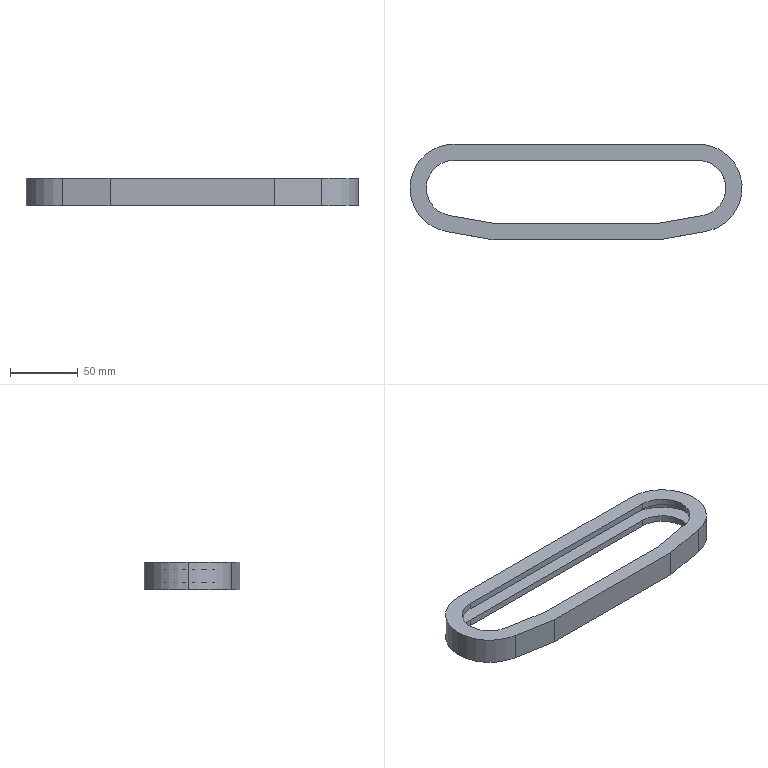Part | SolidWorks | features Extrusion 1, ICE 1 | 1 solid | 32 faces | box 245 x 70.699 x 20 mm | volume 68924 mm3 | plane 20 | cylinder 12 | commonest cylinder face diameters 41 x6 63 x3 65 x3
STEP:
#1=CARTESIAN_POINT('',(121.5,0.,-5.));
#2=VERTEX_POINT('',#1);
#3=CARTESIAN_POINT('',(90.,31.5,-5.));
#4=VERTEX_POINT('',#3);
#5=CARTESIAN_POINT('',(90.,0.,-5.));
#6=DIRECTION('',(0.,0.,1.));
#7=DIRECTION('',(1.,0.,0.));
#8=AXIS2_PLACEMENT_3D('',#5,#6,#7);
#9=CIRCLE('',#8,31.5);
#10=EDGE_CURVE('',#2,#4,#9,.T.);
#11=ORIENTED_EDGE('',*,*,#10,.F.);
#12=CARTESIAN_POINT('',(121.5,0.,5.));
#13=VERTEX_POINT('',#12);
#14=CARTESIAN_POINT('',(121.5,0.,-5.));
#15=DIRECTION('',(0.,0.,1.));
#16=VECTOR('',#15,1000.);
#17=LINE('',#14,#16);
#18=EDGE_CURVE('',#2,#13,#17,.T.);
#19=ORIENTED_EDGE('',*,*,#18,.T.);
#20=CARTESIAN_POINT('',(90.,31.5,5.));
#21=VERTEX_POINT('',#20);
#22=CARTESIAN_POINT('',(90.,0.,5.));
#23=DIRECTION('',(0.,0.,1.));
#24=DIRECTION('',(1.,0.,0.));
#25=AXIS2_PLACEMENT_3D('',#22,#23,#24);
#26=CIRCLE('',#25,31.5);
#27=EDGE_CURVE('',#13,#21,#26,.T.);
#28=ORIENTED_EDGE('',*,*,#27,.T.);
#29=CARTESIAN_POINT('',(90.,31.5,-5.));
#30=DIRECTION('',(0.,0.,1.));
#31=VECTOR('',#30,1000.);
#32=LINE('',#29,#31);
#33=EDGE_CURVE('',#4,#21,#32,.T.);
#34=ORIENTED_EDGE('',*,*,#33,.F.);
#35=EDGE_LOOP('',(#11,#19,#28,#34));
#36=FACE_OUTER_BOUND('',#35,.T.);
#37=CARTESIAN_POINT('',(90.,0.,-5.));
#38=DIRECTION('',(0.,0.,1.));
#39=DIRECTION('',(1.,0.,0.));
#40=AXIS2_PLACEMENT_3D('',#37,#38,#39);
#41=CYLINDRICAL_SURFACE('',#40,31.5);
#42=ADVANCED_FACE('',(#36),#41,.F.);
#43=CARTESIAN_POINT('',(-90.,20.5,10.));
#44=VERTEX_POINT('',#43);
#45=CARTESIAN_POINT('',(-110.5,0.,10.));
#46=VERTEX_POINT('',#45);
#47=CARTESIAN_POINT('',(-90.,0.,10.));
#48=DIRECTION('',(0.,0.,1.));
#49=DIRECTION('',(1.,0.,0.));
#50=AXIS2_PLACEMENT_3D('',#47,#48,#49);
#51=CIRCLE('',#50,20.5);
#52=EDGE_CURVE('',#44,#46,#51,.T.);
#53=ORIENTED_EDGE('',*,*,#52,.T.);
#54=CARTESIAN_POINT('',(-110.5,0.,5.));
#55=VERTEX_POINT('',#54);
#56=CARTESIAN_POINT('',(-110.5,0.,10.));
#57=DIRECTION('',(0.,0.,-1.));
#58=VECTOR('',#57,1000.);
#59=LINE('',#56,#58);
#60=EDGE_CURVE('',#46,#55,#59,.T.);
#61=ORIENTED_EDGE('',*,*,#60,.T.);
#62=CARTESIAN_POINT('',(-90.,20.5,5.));
#63=VERTEX_POINT('',#62);
#64=CARTESIAN_POINT('',(-90.,0.,5.));
#65=DIRECTION('',(0.,0.,1.));
#66=DIRECTION('',(1.,0.,0.));
#67=AXIS2_PLACEMENT_3D('',#64,#65,#66);
#68=CIRCLE('',#67,20.5);
#69=EDGE_CURVE('',#63,#55,#68,.T.);
#70=ORIENTED_EDGE('',*,*,#69,.F.);
#71=CARTESIAN_POINT('',(-90.,20.5,10.));
#72=DIRECTION('',(0.,0.,-1.));
#73=VECTOR('',#72,1000.);
#74=LINE('',#71,#73);
#75=EDGE_CURVE('',#44,#63,#74,.T.);
#76=ORIENTED_EDGE('',*,*,#75,.F.);
#77=EDGE_LOOP('',(#53,#61,#70,#76));
#78=FACE_OUTER_BOUND('',#77,.T.);
#79=CARTESIAN_POINT('',(-90.,0.,10.));
#80=DIRECTION('',(0.,0.,-1.));
#81=DIRECTION('',(-1.,0.,0.));
#82=AXIS2_PLACEMENT_3D('',#79,#80,#81);
#83=CYLINDRICAL_SURFACE('',#82,20.5);
#84=ADVANCED_FACE('',(#78),#83,.F.);
#85=CARTESIAN_POINT('',(-122.5,0.,10.));
#86=VERTEX_POINT('',#85);
#87=CARTESIAN_POINT('',(-95.644,-32.006,10.));
#88=VERTEX_POINT('',#87);
#89=CARTESIAN_POINT('',(-90.,0.,10.));
#90=DIRECTION('',(0.,0.,1.));
#91=DIRECTION('',(1.,0.,0.));
#92=AXIS2_PLACEMENT_3D('',#89,#90,#91);
#93=CIRCLE('',#92,32.5);
#94=EDGE_CURVE('',#86,#88,#93,.T.);
#95=ORIENTED_EDGE('',*,*,#94,.F.);
#96=CARTESIAN_POINT('',(-122.5,0.,-10.));
#97=VERTEX_POINT('',#96);
#98=CARTESIAN_POINT('',(-122.5,0.,10.));
#99=DIRECTION('',(0.,0.,-1.));
#100=VECTOR('',#99,1000.);
#101=LINE('',#98,#100);
#102=EDGE_CURVE('',#86,#97,#101,.T.);
#103=ORIENTED_EDGE('',*,*,#102,.T.);
#104=CARTESIAN_POINT('',(-95.644,-32.006,-10.));
#105=VERTEX_POINT('',#104);
#106=CARTESIAN_POINT('',(-90.,0.,-10.));
#107=DIRECTION('',(0.,0.,1.));
#108=DIRECTION('',(1.,0.,0.));
#109=AXIS2_PLACEMENT_3D('',#106,#107,#108);
#110=CIRCLE('',#109,32.5);
#111=EDGE_CURVE('',#97,#105,#110,.T.);
#112=ORIENTED_EDGE('',*,*,#111,.T.);
#113=CARTESIAN_POINT('',(-95.644,-32.006,10.));
#114=DIRECTION('',(0.,0.,-1.));
#115=VECTOR('',#114,1000.);
#116=LINE('',#113,#115);
#117=EDGE_CURVE('',#88,#105,#116,.T.);
#118=ORIENTED_EDGE('',*,*,#117,.F.);
#119=EDGE_LOOP('',(#95,#103,#112,#118));
#120=FACE_OUTER_BOUND('',#119,.T.);
#121=CARTESIAN_POINT('',(-90.,0.,10.));
#122=DIRECTION('',(0.,0.,-1.));
#123=DIRECTION('',(-1.,0.,0.));
#124=AXIS2_PLACEMENT_3D('',#121,#122,#123);
#125=CYLINDRICAL_SURFACE('',#124,32.5);
#126=ADVANCED_FACE('',(#120),#125,.T.);
#127=CARTESIAN_POINT('',(-90.,20.5,-5.));
#128=VERTEX_POINT('',#127);
#129=CARTESIAN_POINT('',(-110.5,0.,-5.));
#130=VERTEX_POINT('',#129);
#131=CARTESIAN_POINT('',(-90.,0.,-5.));
#132=DIRECTION('',(0.,0.,1.));
#133=DIRECTION('',(1.,0.,0.));
#134=AXIS2_PLACEMENT_3D('',#131,#132,#133);
#135=CIRCLE('',#134,20.5);
#136=EDGE_CURVE('',#128,#130,#135,.T.);
#137=ORIENTED_EDGE('',*,*,#136,.T.);
#138=CARTESIAN_POINT('',(-110.5,0.,-10.));
#139=VERTEX_POINT('',#138);
#140=CARTESIAN_POINT('',(-110.5,0.,10.));
#141=DIRECTION('',(0.,0.,-1.));
#142=VECTOR('',#141,1000.);
#143=LINE('',#140,#142);
#144=EDGE_CURVE('',#130,#139,#143,.T.);
#145=ORIENTED_EDGE('',*,*,#144,.T.);
#146=CARTESIAN_POINT('',(-90.,20.5,-10.));
#147=VERTEX_POINT('',#146);
#148=CARTESIAN_POINT('',(-90.,0.,-10.));
#149=DIRECTION('',(0.,0.,1.));
#150=DIRECTION('',(1.,0.,0.));
#151=AXIS2_PLACEMENT_3D('',#148,#149,#150);
#152=CIRCLE('',#151,20.5);
#153=EDGE_CURVE('',#147,#139,#152,.T.);
#154=ORIENTED_EDGE('',*,*,#153,.F.);
#155=CARTESIAN_POINT('',(-90.,20.5,10.));
#156=DIRECTION('',(0.,0.,-1.));
#157=VECTOR('',#156,1000.);
#158=LINE('',#155,#157);
#159=EDGE_CURVE('',#128,#147,#158,.T.);
#160=ORIENTED_EDGE('',*,*,#159,.F.);
#161=EDGE_LOOP('',(#137,#145,#154,#160));
#162=FACE_OUTER_BOUND('',#161,.T.);
#163=CARTESIAN_POINT('',(-90.,0.,10.));
#164=DIRECTION('',(0.,0.,-1.));
#165=DIRECTION('',(-1.,0.,0.));
#166=AXIS2_PLACEMENT_3D('',#163,#164,#165);
#167=CYLINDRICAL_SURFACE('',#166,20.5);
#168=ADVANCED_FACE('',(#162),#167,.F.);
#169=ORIENTED_EDGE('',*,*,#144,.F.);
#170=CARTESIAN_POINT('',(-93.56,-20.189,-5.));
#171=VERTEX_POINT('',#170);
#172=CARTESIAN_POINT('',(-90.,0.,-5.));
#173=DIRECTION('',(0.,0.,1.));
#174=DIRECTION('',(1.,0.,0.));
#175=AXIS2_PLACEMENT_3D('',#172,#173,#174);
#176=CIRCLE('',#175,20.5);
#177=EDGE_CURVE('',#130,#171,#176,.T.);
#178=ORIENTED_EDGE('',*,*,#177,.T.);
#179=CARTESIAN_POINT('',(-93.56,-20.189,-10.));
#180=VERTEX_POINT('',#179);
#181=CARTESIAN_POINT('',(-93.56,-20.189,10.));
#182=DIRECTION('',(0.,0.,-1.));
#183=VECTOR('',#182,1000.);
#184=LINE('',#181,#183);
#185=EDGE_CURVE('',#171,#180,#184,.T.);
#186=ORIENTED_EDGE('',*,*,#185,.T.);
#187=CARTESIAN_POINT('',(-90.,0.,-10.));
#188=DIRECTION('',(0.,0.,1.));
#189=DIRECTION('',(1.,0.,0.));
#190=AXIS2_PLACEMENT_3D('',#187,#188,#189);
#191=CIRCLE('',#190,20.5);
#192=EDGE_CURVE('',#139,#180,#191,.T.);
#193=ORIENTED_EDGE('',*,*,#192,.F.);
#194=EDGE_LOOP('',(#169,#178,#186,#193));
#195=FACE_OUTER_BOUND('',#194,.T.);
#196=CARTESIAN_POINT('',(-90.,0.,10.));
#197=DIRECTION('',(0.,0.,-1.));
#198=DIRECTION('',(-1.,0.,0.));
#199=AXIS2_PLACEMENT_3D('',#196,#197,#198);
#200=CYLINDRICAL_SURFACE('',#199,20.5);
#201=ADVANCED_FACE('',(#195),#200,.F.);
#202=ORIENTED_EDGE('',*,*,#185,.F.);
#203=CARTESIAN_POINT('',(-59.475,-26.199,-5.));
#204=VERTEX_POINT('',#203);
#205=CARTESIAN_POINT('',(-59.475,-26.199,-5.));
#206=DIRECTION('',(0.9848,-0.1736,0.));
#207=VECTOR('',#206,1000.);
#208=LINE('',#205,#207);
#209=EDGE_CURVE('',#171,#204,#208,.T.);
#210=ORIENTED_EDGE('',*,*,#209,.T.);
#211=CARTESIAN_POINT('',(-59.475,-26.199,-10.));
#212=VERTEX_POINT('',#211);
#213=CARTESIAN_POINT('',(-59.475,-26.199,10.));
#214=DIRECTION('',(0.,0.,-1.));
#215=VECTOR('',#214,1000.);
#216=LINE('',#213,#215);
#217=EDGE_CURVE('',#204,#212,#216,.T.);
#218=ORIENTED_EDGE('',*,*,#217,.T.);
#219=CARTESIAN_POINT('',(-59.475,-26.199,-10.));
#220=DIRECTION('',(0.9848,-0.1736,0.));
#221=VECTOR('',#220,1000.);
#222=LINE('',#219,#221);
#223=EDGE_CURVE('',#180,#212,#222,.T.);
#224=ORIENTED_EDGE('',*,*,#223,.F.);
#225=EDGE_LOOP('',(#202,#210,#218,#224));
#226=FACE_OUTER_BOUND('',#225,.T.);
#227=CARTESIAN_POINT('',(-59.475,-26.199,10.));
#228=DIRECTION('',(0.1736,0.9848,0.));
#229=DIRECTION('',(-0.9848,0.1736,0.));
#230=AXIS2_PLACEMENT_3D('',#227,#228,#229);
#231=PLANE('',#230);
#232=ADVANCED_FACE('',(#226),#231,.T.);
#233=ORIENTED_EDGE('',*,*,#217,.F.);
#234=CARTESIAN_POINT('',(59.475,-26.199,-5.));
#235=VERTEX_POINT('',#234);
#236=CARTESIAN_POINT('',(-59.475,-26.199,-5.));
#237=DIRECTION('',(1.,0.,0.));
#238=VECTOR('',#237,1000.);
#239=LINE('',#236,#238);
#240=EDGE_CURVE('',#204,#235,#239,.T.);
#241=ORIENTED_EDGE('',*,*,#240,.T.);
#242=CARTESIAN_POINT('',(59.475,-26.199,-10.));
#243=VERTEX_POINT('',#242);
#244=CARTESIAN_POINT('',(59.475,-26.199,10.));
#245=DIRECTION('',(0.,0.,-1.));
#246=VECTOR('',#245,1000.);
#247=LINE('',#244,#246);
#248=EDGE_CURVE('',#235,#243,#247,.T.);
#249=ORIENTED_EDGE('',*,*,#248,.T.);
#250=CARTESIAN_POINT('',(-59.475,-26.199,-10.));
#251=DIRECTION('',(1.,0.,0.));
#252=VECTOR('',#251,1000.);
#253=LINE('',#250,#252);
#254=EDGE_CURVE('',#212,#243,#253,.T.);
#255=ORIENTED_EDGE('',*,*,#254,.F.);
#256=EDGE_LOOP('',(#233,#241,#249,#255));
#257=FACE_OUTER_BOUND('',#256,.T.);
#258=CARTESIAN_POINT('',(-59.475,-26.199,10.));
#259=DIRECTION('',(0.,1.,0.));
#260=DIRECTION('',(0.,0.,1.));
#261=AXIS2_PLACEMENT_3D('',#258,#259,#260);
#262=PLANE('',#261);
#263=ADVANCED_FACE('',(#257),#262,.T.);
#264=ORIENTED_EDGE('',*,*,#248,.F.);
#265=CARTESIAN_POINT('',(93.56,-20.189,-5.));
#266=VERTEX_POINT('',#265);
#267=CARTESIAN_POINT('',(59.475,-26.199,-5.));
#268=DIRECTION('',(0.9848,0.1736,0.));
#269=VECTOR('',#268,1000.);
#270=LINE('',#267,#269);
#271=EDGE_CURVE('',#235,#266,#270,.T.);
#272=ORIENTED_EDGE('',*,*,#271,.T.);
#273=CARTESIAN_POINT('',(93.56,-20.189,-10.));
#274=VERTEX_POINT('',#273);
#275=CARTESIAN_POINT('',(93.56,-20.189,10.));
#276=DIRECTION('',(0.,0.,-1.));
#277=VECTOR('',#276,1000.);
#278=LINE('',#275,#277);
#279=EDGE_CURVE('',#266,#274,#278,.T.);
#280=ORIENTED_EDGE('',*,*,#279,.T.);
#281=CARTESIAN_POINT('',(59.475,-26.199,-10.));
#282=DIRECTION('',(0.9848,0.1736,0.));
#283=VECTOR('',#282,1000.);
#284=LINE('',#281,#283);
#285=EDGE_CURVE('',#243,#274,#284,.T.);
#286=ORIENTED_EDGE('',*,*,#285,.F.);
#287=EDGE_LOOP('',(#264,#272,#280,#286));
#288=FACE_OUTER_BOUND('',#287,.T.);
#289=CARTESIAN_POINT('',(59.475,-26.199,10.));
#290=DIRECTION('',(-0.1736,0.9848,0.));
#291=DIRECTION('',(-0.9848,-0.1736,0.));
#292=AXIS2_PLACEMENT_3D('',#289,#290,#291);
#293=PLANE('',#292);
#294=ADVANCED_FACE('',(#288),#293,.T.);
#295=ORIENTED_EDGE('',*,*,#279,.F.);
#296=CARTESIAN_POINT('',(90.,20.5,-5.));
#297=VERTEX_POINT('',#296);
#298=CARTESIAN_POINT('',(90.,0.,-5.));
#299=DIRECTION('',(0.,0.,1.));
#300=DIRECTION('',(1.,0.,0.));
#301=AXIS2_PLACEMENT_3D('',#298,#299,#300);
#302=CIRCLE('',#301,20.5);
#303=EDGE_CURVE('',#266,#297,#302,.T.);
#304=ORIENTED_EDGE('',*,*,#303,.T.);
#305=CARTESIAN_POINT('',(90.,20.5,-10.));
#306=VERTEX_POINT('',#305);
#307=CARTESIAN_POINT('',(90.,20.5,10.));
#308=DIRECTION('',(0.,0.,-1.));
#309=VECTOR('',#308,1000.);
#310=LINE('',#307,#309);
#311=EDGE_CURVE('',#297,#306,#310,.T.);
#312=ORIENTED_EDGE('',*,*,#311,.T.);
#313=CARTESIAN_POINT('',(90.,0.,-10.));
#314=DIRECTION('',(0.,0.,1.));
#315=DIRECTION('',(-1.,0.,0.));
#316=AXIS2_PLACEMENT_3D('',#313,#314,#315);
#317=CIRCLE('',#316,20.5);
#318=EDGE_CURVE('',#274,#306,#317,.T.);
#319=ORIENTED_EDGE('',*,*,#318,.F.);
#320=EDGE_LOOP('',(#295,#304,#312,#319));
#321=FACE_OUTER_BOUND('',#320,.T.);
#322=CARTESIAN_POINT('',(90.,0.,10.));
#323=DIRECTION('',(0.,0.,-1.));
#324=DIRECTION('',(-1.,0.,0.));
#325=AXIS2_PLACEMENT_3D('',#322,#323,#324);
#326=CYLINDRICAL_SURFACE('',#325,20.5);
#327=ADVANCED_FACE('',(#321),#326,.F.);
#328=ORIENTED_EDGE('',*,*,#311,.F.);
#329=CARTESIAN_POINT('',(-90.,20.5,-5.));
#330=DIRECTION('',(-1.,0.,0.));
#331=VECTOR('',#330,1000.);
#332=LINE('',#329,#331);
#333=EDGE_CURVE('',#297,#128,#332,.T.);
#334=ORIENTED_EDGE('',*,*,#333,.T.);
#335=ORIENTED_EDGE('',*,*,#159,.T.);
#336=CARTESIAN_POINT('',(-90.,20.5,-10.));
#337=DIRECTION('',(-1.,0.,0.));
#338=VECTOR('',#337,1000.);
#339=LINE('',#336,#338);
#340=EDGE_CURVE('',#306,#147,#339,.T.);
#341=ORIENTED_EDGE('',*,*,#340,.F.);
#342=EDGE_LOOP('',(#328,#334,#335,#341));
#343=FACE_OUTER_BOUND('',#342,.T.);
#344=CARTESIAN_POINT('',(-90.,20.5,10.));
#345=DIRECTION('',(0.,-1.,0.));
#346=DIRECTION('',(0.,0.,-1.));
#347=AXIS2_PLACEMENT_3D('',#344,#345,#346);
#348=PLANE('',#347);
#349=ADVANCED_FACE('',(#343),#348,.T.);
#350=CARTESIAN_POINT('',(-90.,32.5,10.));
#351=VERTEX_POINT('',#350);
#352=CARTESIAN_POINT('',(-90.,0.,10.));
#353=DIRECTION('',(0.,0.,1.));
#354=DIRECTION('',(1.,0.,0.));
#355=AXIS2_PLACEMENT_3D('',#352,#353,#354);
#356=CIRCLE('',#355,32.5);
#357=EDGE_CURVE('',#351,#86,#356,.T.);
#358=ORIENTED_EDGE('',*,*,#357,.T.);
#359=ORIENTED_EDGE('',*,*,#94,.T.);
#360=CARTESIAN_POINT('',(-60.525,-38.199,10.));
#361=VERTEX_POINT('',#360);
#362=CARTESIAN_POINT('',(-60.525,-38.199,10.));
#363=DIRECTION('',(0.9848,-0.1736,0.));
#364=VECTOR('',#363,1000.);
#365=LINE('',#362,#364);
#366=EDGE_CURVE('',#88,#361,#365,.T.);
#367=ORIENTED_EDGE('',*,*,#366,.T.);
#368=CARTESIAN_POINT('',(60.525,-38.199,10.));
#369=VERTEX_POINT('',#368);
#370=CARTESIAN_POINT('',(-60.525,-38.199,10.));
#371=DIRECTION('',(1.,0.,0.));
#372=VECTOR('',#371,1000.);
#373=LINE('',#370,#372);
#374=EDGE_CURVE('',#361,#369,#373,.T.);
#375=ORIENTED_EDGE('',*,*,#374,.T.);
#376=CARTESIAN_POINT('',(95.644,-32.006,10.));
#377=VERTEX_POINT('',#376);
#378=CARTESIAN_POINT('',(60.525,-38.199,10.));
#379=DIRECTION('',(0.9848,0.1736,0.));
#380=VECTOR('',#379,1000.);
#381=LINE('',#378,#380);
#382=EDGE_CURVE('',#369,#377,#381,.T.);
#383=ORIENTED_EDGE('',*,*,#382,.T.);
#384=CARTESIAN_POINT('',(90.,32.5,10.));
#385=VERTEX_POINT('',#384);
#386=CARTESIAN_POINT('',(90.,0.,10.));
#387=DIRECTION('',(0.,0.,1.));
#388=DIRECTION('',(-1.,0.,0.));
#389=AXIS2_PLACEMENT_3D('',#386,#387,#388);
#390=CIRCLE('',#389,32.5);
#391=EDGE_CURVE('',#377,#385,#390,.T.);
#392=ORIENTED_EDGE('',*,*,#391,.T.);
#393=CARTESIAN_POINT('',(-90.,32.5,10.));
#394=DIRECTION('',(-1.,0.,0.));
#395=VECTOR('',#394,1000.);
#396=LINE('',#393,#395);
#397=EDGE_CURVE('',#385,#351,#396,.T.);
#398=ORIENTED_EDGE('',*,*,#397,.T.);
#399=EDGE_LOOP('',(#358,#359,#367,#375,#383,#392,#398));
#400=FACE_OUTER_BOUND('',#399,.T.);
#401=CARTESIAN_POINT('',(-93.56,-20.189,10.));
#402=VERTEX_POINT('',#401);
#403=CARTESIAN_POINT('',(-59.475,-26.199,10.));
#404=VERTEX_POINT('',#403);
#405=CARTESIAN_POINT('',(-59.475,-26.199,10.));
#406=DIRECTION('',(0.9848,-0.1736,0.));
#407=VECTOR('',#406,1000.);
#408=LINE('',#405,#407);
#409=EDGE_CURVE('',#402,#404,#408,.T.);
#410=ORIENTED_EDGE('',*,*,#409,.F.);
#411=CARTESIAN_POINT('',(-90.,0.,10.));
#412=DIRECTION('',(0.,0.,1.));
#413=DIRECTION('',(1.,0.,0.));
#414=AXIS2_PLACEMENT_3D('',#411,#412,#413);
#415=CIRCLE('',#414,20.5);
#416=EDGE_CURVE('',#46,#402,#415,.T.);
#417=ORIENTED_EDGE('',*,*,#416,.F.);
#418=ORIENTED_EDGE('',*,*,#52,.F.);
#419=CARTESIAN_POINT('',(90.,20.5,10.));
#420=VERTEX_POINT('',#419);
#421=CARTESIAN_POINT('',(-90.,20.5,10.));
#422=DIRECTION('',(-1.,0.,0.));
#423=VECTOR('',#422,1000.);
#424=LINE('',#421,#423);
#425=EDGE_CURVE('',#420,#44,#424,.T.);
#426=ORIENTED_EDGE('',*,*,#425,.F.);
#427=CARTESIAN_POINT('',(93.56,-20.189,10.));
#428=VERTEX_POINT('',#427);
#429=CARTESIAN_POINT('',(90.,0.,10.));
#430=DIRECTION('',(0.,0.,1.));
#431=DIRECTION('',(-1.,0.,0.));
#432=AXIS2_PLACEMENT_3D('',#429,#430,#431);
#433=CIRCLE('',#432,20.5);
#434=EDGE_CURVE('',#428,#420,#433,.T.);
#435=ORIENTED_EDGE('',*,*,#434,.F.);
#436=CARTESIAN_POINT('',(59.475,-26.199,10.));
#437=VERTEX_POINT('',#436);
#438=CARTESIAN_POINT('',(59.475,-26.199,10.));
#439=DIRECTION('',(0.9848,0.1736,0.));
#440=VECTOR('',#439,1000.);
#441=LINE('',#438,#440);
#442=EDGE_CURVE('',#437,#428,#441,.T.);
#443=ORIENTED_EDGE('',*,*,#442,.F.);
#444=CARTESIAN_POINT('',(-59.475,-26.199,10.));
#445=DIRECTION('',(1.,0.,0.));
#446=VECTOR('',#445,1000.);
#447=LINE('',#444,#446);
#448=EDGE_CURVE('',#404,#437,#447,.T.);
#449=ORIENTED_EDGE('',*,*,#448,.F.);
#450=EDGE_LOOP('',(#410,#417,#418,#426,#435,#443,#449));
#451=FACE_BOUND('',#450,.T.);
#452=CARTESIAN_POINT('',(-90.,0.,10.));
#453=DIRECTION('',(0.,0.,1.));
#454=DIRECTION('',(1.,0.,0.));
#455=AXIS2_PLACEMENT_3D('',#452,#453,#454);
#456=PLANE('',#455);
#457=ADVANCED_FACE('',(#400,#451),#456,.T.);
#458=CARTESIAN_POINT('',(-90.,32.5,-10.));
#459=VERTEX_POINT('',#458);
#460=CARTESIAN_POINT('',(-90.,0.,-10.));
#461=DIRECTION('',(0.,0.,1.));
#462=DIRECTION('',(1.,0.,0.));
#463=AXIS2_PLACEMENT_3D('',#460,#461,#462);
#464=CIRCLE('',#463,32.5);
#465=EDGE_CURVE('',#459,#97,#464,.T.);
#466=ORIENTED_EDGE('',*,*,#465,.F.);
#467=CARTESIAN_POINT('',(90.,32.5,-10.));
#468=VERTEX_POINT('',#467);
#469=CARTESIAN_POINT('',(-90.,32.5,-10.));
#470=DIRECTION('',(-1.,0.,0.));
#471=VECTOR('',#470,1000.);
#472=LINE('',#469,#471);
#473=EDGE_CURVE('',#468,#459,#472,.T.);
#474=ORIENTED_EDGE('',*,*,#473,.F.);
#475=CARTESIAN_POINT('',(95.644,-32.006,-10.));
#476=VERTEX_POINT('',#475);
#477=CARTESIAN_POINT('',(90.,0.,-10.));
#478=DIRECTION('',(0.,0.,1.));
#479=DIRECTION('',(-1.,0.,0.));
#480=AXIS2_PLACEMENT_3D('',#477,#478,#479);
#481=CIRCLE('',#480,32.5);
#482=EDGE_CURVE('',#476,#468,#481,.T.);
#483=ORIENTED_EDGE('',*,*,#482,.F.);
#484=CARTESIAN_POINT('',(60.525,-38.199,-10.));
#485=VERTEX_POINT('',#484);
#486=CARTESIAN_POINT('',(60.525,-38.199,-10.));
#487=DIRECTION('',(0.9848,0.1736,0.));
#488=VECTOR('',#487,1000.);
#489=LINE('',#486,#488);
#490=EDGE_CURVE('',#485,#476,#489,.T.);
#491=ORIENTED_EDGE('',*,*,#490,.F.);
#492=CARTESIAN_POINT('',(-60.525,-38.199,-10.));
#493=VERTEX_POINT('',#492);
#494=CARTESIAN_POINT('',(-60.525,-38.199,-10.));
#495=DIRECTION('',(1.,0.,0.));
#496=VECTOR('',#495,1000.);
#497=LINE('',#494,#496);
#498=EDGE_CURVE('',#493,#485,#497,.T.);
#499=ORIENTED_EDGE('',*,*,#498,.F.);
#500=CARTESIAN_POINT('',(-60.525,-38.199,-10.));
#501=DIRECTION('',(0.9848,-0.1736,0.));
#502=VECTOR('',#501,1000.);
#503=LINE('',#500,#502);
#504=EDGE_CURVE('',#105,#493,#503,.T.);
#505=ORIENTED_EDGE('',*,*,#504,.F.);
#506=ORIENTED_EDGE('',*,*,#111,.F.);
#507=EDGE_LOOP('',(#466,#474,#483,#491,#499,#505,#506));
#508=FACE_OUTER_BOUND('',#507,.T.);
#509=ORIENTED_EDGE('',*,*,#153,.T.);
#510=ORIENTED_EDGE('',*,*,#192,.T.);
#511=ORIENTED_EDGE('',*,*,#223,.T.);
#512=ORIENTED_EDGE('',*,*,#254,.T.);
#513=ORIENTED_EDGE('',*,*,#285,.T.);
#514=ORIENTED_EDGE('',*,*,#318,.T.);
#515=ORIENTED_EDGE('',*,*,#340,.T.);
#516=EDGE_LOOP('',(#509,#510,#511,#512,#513,#514,#515));
#517=FACE_BOUND('',#516,.T.);
#518=CARTESIAN_POINT('',(-90.,0.,-10.));
#519=DIRECTION('',(0.,0.,1.));
#520=DIRECTION('',(1.,0.,0.));
#521=AXIS2_PLACEMENT_3D('',#518,#519,#520);
#522=PLANE('',#521);
#523=ADVANCED_FACE('',(#508,#517),#522,.F.);
#524=ORIENTED_EDGE('',*,*,#102,.F.);
#525=ORIENTED_EDGE('',*,*,#357,.F.);
#526=CARTESIAN_POINT('',(-90.,32.5,10.));
#527=DIRECTION('',(0.,0.,-1.));
#528=VECTOR('',#527,1000.);
#529=LINE('',#526,#528);
#530=EDGE_CURVE('',#351,#459,#529,.T.);
#531=ORIENTED_EDGE('',*,*,#530,.T.);
#532=ORIENTED_EDGE('',*,*,#465,.T.);
#533=EDGE_LOOP('',(#524,#525,#531,#532));
#534=FACE_OUTER_BOUND('',#533,.T.);
#535=CARTESIAN_POINT('',(-90.,0.,10.));
#536=DIRECTION('',(0.,0.,-1.));
#537=DIRECTION('',(-1.,0.,0.));
#538=AXIS2_PLACEMENT_3D('',#535,#536,#537);
#539=CYLINDRICAL_SURFACE('',#538,32.5);
#540=ADVANCED_FACE('',(#534),#539,.T.);
#541=ORIENTED_EDGE('',*,*,#504,.T.);
#542=CARTESIAN_POINT('',(-60.525,-38.199,10.));
#543=DIRECTION('',(0.,0.,-1.));
#544=VECTOR('',#543,1000.);
#545=LINE('',#542,#544);
#546=EDGE_CURVE('',#361,#493,#545,.T.);
#547=ORIENTED_EDGE('',*,*,#546,.F.);
#548=ORIENTED_EDGE('',*,*,#366,.F.);
#549=ORIENTED_EDGE('',*,*,#117,.T.);
#550=EDGE_LOOP('',(#541,#547,#548,#549));
#551=FACE_OUTER_BOUND('',#550,.T.);
#552=CARTESIAN_POINT('',(-60.525,-38.199,10.));
#553=DIRECTION('',(0.1736,0.9848,0.));
#554=DIRECTION('',(-0.9848,0.1736,0.));
#555=AXIS2_PLACEMENT_3D('',#552,#553,#554);
#556=PLANE('',#555);
#557=ADVANCED_FACE('',(#551),#556,.F.);
#558=ORIENTED_EDGE('',*,*,#498,.T.);
#559=CARTESIAN_POINT('',(60.525,-38.199,10.));
#560=DIRECTION('',(0.,0.,-1.));
#561=VECTOR('',#560,1000.);
#562=LINE('',#559,#561);
#563=EDGE_CURVE('',#369,#485,#562,.T.);
#564=ORIENTED_EDGE('',*,*,#563,.F.);
#565=ORIENTED_EDGE('',*,*,#374,.F.);
#566=ORIENTED_EDGE('',*,*,#546,.T.);
#567=EDGE_LOOP('',(#558,#564,#565,#566));
#568=FACE_OUTER_BOUND('',#567,.T.);
#569=CARTESIAN_POINT('',(-60.525,-38.199,10.));
#570=DIRECTION('',(0.,1.,0.));
#571=DIRECTION('',(0.,0.,1.));
#572=AXIS2_PLACEMENT_3D('',#569,#570,#571);
#573=PLANE('',#572);
#574=ADVANCED_FACE('',(#568),#573,.F.);
#575=ORIENTED_EDGE('',*,*,#490,.T.);
#576=CARTESIAN_POINT('',(95.644,-32.006,10.));
#577=DIRECTION('',(0.,0.,-1.));
#578=VECTOR('',#577,1000.);
#579=LINE('',#576,#578);
#580=EDGE_CURVE('',#377,#476,#579,.T.);
#581=ORIENTED_EDGE('',*,*,#580,.F.);
#582=ORIENTED_EDGE('',*,*,#382,.F.);
#583=ORIENTED_EDGE('',*,*,#563,.T.);
#584=EDGE_LOOP('',(#575,#581,#582,#583));
#585=FACE_OUTER_BOUND('',#584,.T.);
#586=CARTESIAN_POINT('',(60.525,-38.199,10.));
#587=DIRECTION('',(-0.1736,0.9848,0.));
#588=DIRECTION('',(-0.9848,-0.1736,0.));
#589=AXIS2_PLACEMENT_3D('',#586,#587,#588);
#590=PLANE('',#589);
#591=ADVANCED_FACE('',(#585),#590,.F.);
#592=ORIENTED_EDGE('',*,*,#482,.T.);
#593=CARTESIAN_POINT('',(90.,32.5,10.));
#594=DIRECTION('',(0.,0.,-1.));
#595=VECTOR('',#594,1000.);
#596=LINE('',#593,#595);
#597=EDGE_CURVE('',#385,#468,#596,.T.);
#598=ORIENTED_EDGE('',*,*,#597,.F.);
#599=ORIENTED_EDGE('',*,*,#391,.F.);
#600=ORIENTED_EDGE('',*,*,#580,.T.);
#601=EDGE_LOOP('',(#592,#598,#599,#600));
#602=FACE_OUTER_BOUND('',#601,.T.);
#603=CARTESIAN_POINT('',(90.,0.,10.));
#604=DIRECTION('',(0.,0.,-1.));
#605=DIRECTION('',(-1.,0.,0.));
#606=AXIS2_PLACEMENT_3D('',#603,#604,#605);
#607=CYLINDRICAL_SURFACE('',#606,32.5);
#608=ADVANCED_FACE('',(#602),#607,.T.);
#609=ORIENTED_EDGE('',*,*,#473,.T.);
#610=ORIENTED_EDGE('',*,*,#530,.F.);
#611=ORIENTED_EDGE('',*,*,#397,.F.);
#612=ORIENTED_EDGE('',*,*,#597,.T.);
#613=EDGE_LOOP('',(#609,#610,#611,#612));
#614=FACE_OUTER_BOUND('',#613,.T.);
#615=CARTESIAN_POINT('',(-90.,32.5,10.));
#616=DIRECTION('',(0.,-1.,0.));
#617=DIRECTION('',(0.,0.,-1.));
#618=AXIS2_PLACEMENT_3D('',#615,#616,#617);
#619=PLANE('',#618);
#620=ADVANCED_FACE('',(#614),#619,.F.);
#621=ORIENTED_EDGE('',*,*,#60,.F.);
#622=ORIENTED_EDGE('',*,*,#416,.T.);
#623=CARTESIAN_POINT('',(-93.56,-20.189,5.));
#624=VERTEX_POINT('',#623);
#625=CARTESIAN_POINT('',(-93.56,-20.189,10.));
#626=DIRECTION('',(0.,0.,-1.));
#627=VECTOR('',#626,1000.);
#628=LINE('',#625,#627);
#629=EDGE_CURVE('',#402,#624,#628,.T.);
#630=ORIENTED_EDGE('',*,*,#629,.T.);
#631=CARTESIAN_POINT('',(-90.,0.,5.));
#632=DIRECTION('',(0.,0.,1.));
#633=DIRECTION('',(1.,0.,0.));
#634=AXIS2_PLACEMENT_3D('',#631,#632,#633);
#635=CIRCLE('',#634,20.5);
#636=EDGE_CURVE('',#55,#624,#635,.T.);
#637=ORIENTED_EDGE('',*,*,#636,.F.);
#638=EDGE_LOOP('',(#621,#622,#630,#637));
#639=FACE_OUTER_BOUND('',#638,.T.);
#640=CARTESIAN_POINT('',(-90.,0.,10.));
#641=DIRECTION('',(0.,0.,-1.));
#642=DIRECTION('',(-1.,0.,0.));
#643=AXIS2_PLACEMENT_3D('',#640,#641,#642);
#644=CYLINDRICAL_SURFACE('',#643,20.5);
#645=ADVANCED_FACE('',(#639),#644,.F.);
#646=CARTESIAN_POINT('',(-59.475,-26.199,5.));
#647=VERTEX_POINT('',#646);
#648=CARTESIAN_POINT('',(-59.475,-26.199,5.));
#649=DIRECTION('',(0.9848,-0.1736,0.));
#650=VECTOR('',#649,1000.);
#651=LINE('',#648,#650);
#652=EDGE_CURVE('',#624,#647,#651,.T.);
#653=ORIENTED_EDGE('',*,*,#652,.F.);
#654=ORIENTED_EDGE('',*,*,#629,.F.);
#655=ORIENTED_EDGE('',*,*,#409,.T.);
#656=CARTESIAN_POINT('',(-59.475,-26.199,10.));
#657=DIRECTION('',(0.,0.,-1.));
#658=VECTOR('',#657,1000.);
#659=LINE('',#656,#658);
#660=EDGE_CURVE('',#404,#647,#659,.T.);
#661=ORIENTED_EDGE('',*,*,#660,.T.);
#662=EDGE_LOOP('',(#653,#654,#655,#661));
#663=FACE_OUTER_BOUND('',#662,.T.);
#664=CARTESIAN_POINT('',(-59.475,-26.199,10.));
#665=DIRECTION('',(0.1736,0.9848,0.));
#666=DIRECTION('',(-0.9848,0.1736,0.));
#667=AXIS2_PLACEMENT_3D('',#664,#665,#666);
#668=PLANE('',#667);
#669=ADVANCED_FACE('',(#663),#668,.T.);
#670=CARTESIAN_POINT('',(59.475,-26.199,5.));
#671=VERTEX_POINT('',#670);
#672=CARTESIAN_POINT('',(-59.475,-26.199,5.));
#673=DIRECTION('',(1.,0.,0.));
#674=VECTOR('',#673,1000.);
#675=LINE('',#672,#674);
#676=EDGE_CURVE('',#647,#671,#675,.T.);
#677=ORIENTED_EDGE('',*,*,#676,.F.);
#678=ORIENTED_EDGE('',*,*,#660,.F.);
#679=ORIENTED_EDGE('',*,*,#448,.T.);
#680=CARTESIAN_POINT('',(59.475,-26.199,10.));
#681=DIRECTION('',(0.,0.,-1.));
#682=VECTOR('',#681,1000.);
#683=LINE('',#680,#682);
#684=EDGE_CURVE('',#437,#671,#683,.T.);
#685=ORIENTED_EDGE('',*,*,#684,.T.);
#686=EDGE_LOOP('',(#677,#678,#679,#685));
#687=FACE_OUTER_BOUND('',#686,.T.);
#688=CARTESIAN_POINT('',(-59.475,-26.199,10.));
#689=DIRECTION('',(0.,1.,0.));
#690=DIRECTION('',(0.,0.,1.));
#691=AXIS2_PLACEMENT_3D('',#688,#689,#690);
#692=PLANE('',#691);
#693=ADVANCED_FACE('',(#687),#692,.T.);
#694=CARTESIAN_POINT('',(93.56,-20.189,5.));
#695=VERTEX_POINT('',#694);
#696=CARTESIAN_POINT('',(59.475,-26.199,5.));
#697=DIRECTION('',(0.9848,0.1736,0.));
#698=VECTOR('',#697,1000.);
#699=LINE('',#696,#698);
#700=EDGE_CURVE('',#671,#695,#699,.T.);
#701=ORIENTED_EDGE('',*,*,#700,.F.);
#702=ORIENTED_EDGE('',*,*,#684,.F.);
#703=ORIENTED_EDGE('',*,*,#442,.T.);
#704=CARTESIAN_POINT('',(93.56,-20.189,10.));
#705=DIRECTION('',(0.,0.,-1.));
#706=VECTOR('',#705,1000.);
#707=LINE('',#704,#706);
#708=EDGE_CURVE('',#428,#695,#707,.T.);
#709=ORIENTED_EDGE('',*,*,#708,.T.);
#710=EDGE_LOOP('',(#701,#702,#703,#709));
#711=FACE_OUTER_BOUND('',#710,.T.);
#712=CARTESIAN_POINT('',(59.475,-26.199,10.));
#713=DIRECTION('',(-0.1736,0.9848,0.));
#714=DIRECTION('',(-0.9848,-0.1736,0.));
#715=AXIS2_PLACEMENT_3D('',#712,#713,#714);
#716=PLANE('',#715);
#717=ADVANCED_FACE('',(#711),#716,.T.);
#718=CARTESIAN_POINT('',(90.,20.5,5.));
#719=VERTEX_POINT('',#718);
#720=CARTESIAN_POINT('',(90.,0.,5.));
#721=DIRECTION('',(0.,0.,1.));
#722=DIRECTION('',(1.,0.,0.));
#723=AXIS2_PLACEMENT_3D('',#720,#721,#722);
#724=CIRCLE('',#723,20.5);
#725=EDGE_CURVE('',#695,#719,#724,.T.);
#726=ORIENTED_EDGE('',*,*,#725,.F.);
#727=ORIENTED_EDGE('',*,*,#708,.F.);
#728=ORIENTED_EDGE('',*,*,#434,.T.);
#729=CARTESIAN_POINT('',(90.,20.5,10.));
#730=DIRECTION('',(0.,0.,-1.));
#731=VECTOR('',#730,1000.);
#732=LINE('',#729,#731);
#733=EDGE_CURVE('',#420,#719,#732,.T.);
#734=ORIENTED_EDGE('',*,*,#733,.T.);
#735=EDGE_LOOP('',(#726,#727,#728,#734));
#736=FACE_OUTER_BOUND('',#735,.T.);
#737=CARTESIAN_POINT('',(90.,0.,10.));
#738=DIRECTION('',(0.,0.,-1.));
#739=DIRECTION('',(-1.,0.,0.));
#740=AXIS2_PLACEMENT_3D('',#737,#738,#739);
#741=CYLINDRICAL_SURFACE('',#740,20.5);
#742=ADVANCED_FACE('',(#736),#741,.F.);
#743=CARTESIAN_POINT('',(-90.,20.5,5.));
#744=DIRECTION('',(-1.,0.,0.));
#745=VECTOR('',#744,1000.);
#746=LINE('',#743,#745);
#747=EDGE_CURVE('',#719,#63,#746,.T.);
#748=ORIENTED_EDGE('',*,*,#747,.F.);
#749=ORIENTED_EDGE('',*,*,#733,.F.);
#750=ORIENTED_EDGE('',*,*,#425,.T.);
#751=ORIENTED_EDGE('',*,*,#75,.T.);
#752=EDGE_LOOP('',(#748,#749,#750,#751));
#753=FACE_OUTER_BOUND('',#752,.T.);
#754=CARTESIAN_POINT('',(-90.,20.5,10.));
#755=DIRECTION('',(0.,-1.,0.));
#756=DIRECTION('',(0.,0.,-1.));
#757=AXIS2_PLACEMENT_3D('',#754,#755,#756);
#758=PLANE('',#757);
#759=ADVANCED_FACE('',(#753),#758,.T.);
#760=CARTESIAN_POINT('',(-60.437,-37.199,5.));
#761=VERTEX_POINT('',#760);
#762=CARTESIAN_POINT('',(60.437,-37.199,5.));
#763=VERTEX_POINT('',#762);
#764=CARTESIAN_POINT('',(-60.437,-37.199,5.));
#765=DIRECTION('',(1.,0.,0.));
#766=VECTOR('',#765,1000.);
#767=LINE('',#764,#766);
#768=EDGE_CURVE('',#761,#763,#767,.T.);
#769=ORIENTED_EDGE('',*,*,#768,.T.);
#770=CARTESIAN_POINT('',(60.437,-37.199,-5.));
#771=VERTEX_POINT('',#770);
#772=CARTESIAN_POINT('',(60.437,-37.199,-5.));
#773=DIRECTION('',(0.,0.,1.));
#774=VECTOR('',#773,1000.);
#775=LINE('',#772,#774);
#776=EDGE_CURVE('',#771,#763,#775,.T.);
#777=ORIENTED_EDGE('',*,*,#776,.F.);
#778=CARTESIAN_POINT('',(-60.437,-37.199,-5.));
#779=VERTEX_POINT('',#778);
#780=CARTESIAN_POINT('',(-60.437,-37.199,-5.));
#781=DIRECTION('',(1.,0.,0.));
#782=VECTOR('',#781,1000.);
#783=LINE('',#780,#782);
#784=EDGE_CURVE('',#779,#771,#783,.T.);
#785=ORIENTED_EDGE('',*,*,#784,.F.);
#786=CARTESIAN_POINT('',(-60.437,-37.199,-5.));
#787=DIRECTION('',(0.,0.,1.));
#788=VECTOR('',#787,1000.);
#789=LINE('',#786,#788);
#790=EDGE_CURVE('',#779,#761,#789,.T.);
#791=ORIENTED_EDGE('',*,*,#790,.T.);
#792=EDGE_LOOP('',(#769,#777,#785,#791));
#793=FACE_OUTER_BOUND('',#792,.T.);
#794=CARTESIAN_POINT('',(-60.437,-37.199,-5.));
#795=DIRECTION('',(0.,-1.,0.));
#796=DIRECTION('',(0.,0.,-1.));
#797=AXIS2_PLACEMENT_3D('',#794,#795,#796);
#798=PLANE('',#797);
#799=ADVANCED_FACE('',(#793),#798,.F.);
#800=CARTESIAN_POINT('',(-95.47,-31.021,5.));
#801=VERTEX_POINT('',#800);
#802=CARTESIAN_POINT('',(-95.47,-31.021,5.));
#803=DIRECTION('',(0.9848,-0.1736,0.));
#804=VECTOR('',#803,1000.);
#805=LINE('',#802,#804);
#806=EDGE_CURVE('',#801,#761,#805,.T.);
#807=ORIENTED_EDGE('',*,*,#806,.T.);
#808=ORIENTED_EDGE('',*,*,#790,.F.);
#809=CARTESIAN_POINT('',(-95.47,-31.021,-5.));
#810=VERTEX_POINT('',#809);
#811=CARTESIAN_POINT('',(-95.47,-31.021,-5.));
#812=DIRECTION('',(0.9848,-0.1736,0.));
#813=VECTOR('',#812,1000.);
#814=LINE('',#811,#813);
#815=EDGE_CURVE('',#810,#779,#814,.T.);
#816=ORIENTED_EDGE('',*,*,#815,.F.);
#817=CARTESIAN_POINT('',(-95.47,-31.021,-5.));
#818=DIRECTION('',(0.,0.,1.));
#819=VECTOR('',#818,1000.);
#820=LINE('',#817,#819);
#821=EDGE_CURVE('',#810,#801,#820,.T.);
#822=ORIENTED_EDGE('',*,*,#821,.T.);
#823=EDGE_LOOP('',(#807,#808,#816,#822));
#824=FACE_OUTER_BOUND('',#823,.T.);
#825=CARTESIAN_POINT('',(-95.47,-31.021,-5.));
#826=DIRECTION('',(-0.1736,-0.9848,0.));
#827=DIRECTION('',(0.9848,-0.1736,0.));
#828=AXIS2_PLACEMENT_3D('',#825,#826,#827);
#829=PLANE('',#828);
#830=ADVANCED_FACE('',(#824),#829,.F.);
#831=CARTESIAN_POINT('',(-90.,31.5,5.));
#832=VERTEX_POINT('',#831);
#833=CARTESIAN_POINT('',(-90.,0.,5.));
#834=DIRECTION('',(0.,0.,1.));
#835=DIRECTION('',(1.,0.,0.));
#836=AXIS2_PLACEMENT_3D('',#833,#834,#835);
#837=CIRCLE('',#836,31.5);
#838=EDGE_CURVE('',#832,#801,#837,.T.);
#839=ORIENTED_EDGE('',*,*,#838,.T.);
#840=ORIENTED_EDGE('',*,*,#821,.F.);
#841=CARTESIAN_POINT('',(-90.,31.5,-5.));
#842=VERTEX_POINT('',#841);
#843=CARTESIAN_POINT('',(-90.,0.,-5.));
#844=DIRECTION('',(0.,0.,1.));
#845=DIRECTION('',(1.,0.,0.));
#846=AXIS2_PLACEMENT_3D('',#843,#844,#845);
#847=CIRCLE('',#846,31.5);
#848=EDGE_CURVE('',#842,#810,#847,.T.);
#849=ORIENTED_EDGE('',*,*,#848,.F.);
#850=CARTESIAN_POINT('',(-90.,31.5,-5.));
#851=DIRECTION('',(0.,0.,1.));
#852=VECTOR('',#851,1000.);
#853=LINE('',#850,#852);
#854=EDGE_CURVE('',#842,#832,#853,.T.);
#855=ORIENTED_EDGE('',*,*,#854,.T.);
#856=EDGE_LOOP('',(#839,#840,#849,#855));
#857=FACE_OUTER_BOUND('',#856,.T.);
#858=CARTESIAN_POINT('',(-90.,0.,-5.));
#859=DIRECTION('',(0.,0.,1.));
#860=DIRECTION('',(1.,0.,0.));
#861=AXIS2_PLACEMENT_3D('',#858,#859,#860);
#862=CYLINDRICAL_SURFACE('',#861,31.5);
#863=ADVANCED_FACE('',(#857),#862,.F.);
#864=CARTESIAN_POINT('',(90.,31.5,5.));
#865=DIRECTION('',(-1.,0.,0.));
#866=VECTOR('',#865,1000.);
#867=LINE('',#864,#866);
#868=EDGE_CURVE('',#21,#832,#867,.T.);
#869=ORIENTED_EDGE('',*,*,#868,.T.);
#870=ORIENTED_EDGE('',*,*,#854,.F.);
#871=CARTESIAN_POINT('',(90.,31.5,-5.));
#872=DIRECTION('',(-1.,0.,0.));
#873=VECTOR('',#872,1000.);
#874=LINE('',#871,#873);
#875=EDGE_CURVE('',#4,#842,#874,.T.);
#876=ORIENTED_EDGE('',*,*,#875,.F.);
#877=ORIENTED_EDGE('',*,*,#33,.T.);
#878=EDGE_LOOP('',(#869,#870,#876,#877));
#879=FACE_OUTER_BOUND('',#878,.T.);
#880=CARTESIAN_POINT('',(90.,31.5,-5.));
#881=DIRECTION('',(0.,1.,0.));
#882=DIRECTION('',(0.,0.,1.));
#883=AXIS2_PLACEMENT_3D('',#880,#881,#882);
#884=PLANE('',#883);
#885=ADVANCED_FACE('',(#879),#884,.F.);
#886=ORIENTED_EDGE('',*,*,#18,.F.);
#887=CARTESIAN_POINT('',(95.47,-31.021,-5.));
#888=VERTEX_POINT('',#887);
#889=CARTESIAN_POINT('',(90.,0.,-5.));
#890=DIRECTION('',(0.,0.,1.));
#891=DIRECTION('',(1.,0.,0.));
#892=AXIS2_PLACEMENT_3D('',#889,#890,#891);
#893=CIRCLE('',#892,31.5);
#894=EDGE_CURVE('',#888,#2,#893,.T.);
#895=ORIENTED_EDGE('',*,*,#894,.F.);
#896=CARTESIAN_POINT('',(95.47,-31.021,5.));
#897=VERTEX_POINT('',#896);
#898=CARTESIAN_POINT('',(95.47,-31.021,-5.));
#899=DIRECTION('',(0.,0.,1.));
#900=VECTOR('',#899,1000.);
#901=LINE('',#898,#900);
#902=EDGE_CURVE('',#888,#897,#901,.T.);
#903=ORIENTED_EDGE('',*,*,#902,.T.);
#904=CARTESIAN_POINT('',(90.,0.,5.));
#905=DIRECTION('',(0.,0.,1.));
#906=DIRECTION('',(1.,0.,0.));
#907=AXIS2_PLACEMENT_3D('',#904,#905,#906);
#908=CIRCLE('',#907,31.5);
#909=EDGE_CURVE('',#897,#13,#908,.T.);
#910=ORIENTED_EDGE('',*,*,#909,.T.);
#911=EDGE_LOOP('',(#886,#895,#903,#910));
#912=FACE_OUTER_BOUND('',#911,.T.);
#913=CARTESIAN_POINT('',(90.,0.,-5.));
#914=DIRECTION('',(0.,0.,1.));
#915=DIRECTION('',(1.,0.,0.));
#916=AXIS2_PLACEMENT_3D('',#913,#914,#915);
#917=CYLINDRICAL_SURFACE('',#916,31.5);
#918=ADVANCED_FACE('',(#912),#917,.F.);
#919=CARTESIAN_POINT('',(60.437,-37.199,5.));
#920=DIRECTION('',(0.9848,0.1736,0.));
#921=VECTOR('',#920,1000.);
#922=LINE('',#919,#921);
#923=EDGE_CURVE('',#763,#897,#922,.T.);
#924=ORIENTED_EDGE('',*,*,#923,.T.);
#925=ORIENTED_EDGE('',*,*,#902,.F.);
#926=CARTESIAN_POINT('',(60.437,-37.199,-5.));
#927=DIRECTION('',(0.9848,0.1736,0.));
#928=VECTOR('',#927,1000.);
#929=LINE('',#926,#928);
#930=EDGE_CURVE('',#771,#888,#929,.T.);
#931=ORIENTED_EDGE('',*,*,#930,.F.);
#932=ORIENTED_EDGE('',*,*,#776,.T.);
#933=EDGE_LOOP('',(#924,#925,#931,#932));
#934=FACE_OUTER_BOUND('',#933,.T.);
#935=CARTESIAN_POINT('',(60.437,-37.199,-5.));
#936=DIRECTION('',(0.1736,-0.9848,0.));
#937=DIRECTION('',(0.9848,0.1736,0.));
#938=AXIS2_PLACEMENT_3D('',#935,#936,#937);
#939=PLANE('',#938);
#940=ADVANCED_FACE('',(#934),#939,.F.);
#941=ORIENTED_EDGE('',*,*,#333,.F.);
#942=ORIENTED_EDGE('',*,*,#303,.F.);
#943=ORIENTED_EDGE('',*,*,#271,.F.);
#944=ORIENTED_EDGE('',*,*,#240,.F.);
#945=ORIENTED_EDGE('',*,*,#209,.F.);
#946=ORIENTED_EDGE('',*,*,#177,.F.);
#947=ORIENTED_EDGE('',*,*,#136,.F.);
#948=EDGE_LOOP('',(#941,#942,#943,#944,#945,#946,#947));
#949=FACE_BOUND('',#948,.T.);
#950=ORIENTED_EDGE('',*,*,#784,.T.);
#951=ORIENTED_EDGE('',*,*,#930,.T.);
#952=ORIENTED_EDGE('',*,*,#894,.T.);
#953=ORIENTED_EDGE('',*,*,#10,.T.);
#954=ORIENTED_EDGE('',*,*,#875,.T.);
#955=ORIENTED_EDGE('',*,*,#848,.T.);
#956=ORIENTED_EDGE('',*,*,#815,.T.);
#957=EDGE_LOOP('',(#950,#951,#952,#953,#954,#955,#956));
#958=FACE_OUTER_BOUND('',#957,.T.);
#959=CARTESIAN_POINT('',(90.,0.,-5.));
#960=DIRECTION('',(0.,0.,1.));
#961=DIRECTION('',(1.,0.,0.));
#962=AXIS2_PLACEMENT_3D('',#959,#960,#961);
#963=PLANE('',#962);
#964=ADVANCED_FACE('',(#949,#958),#963,.T.);
#965=ORIENTED_EDGE('',*,*,#69,.T.);
#966=ORIENTED_EDGE('',*,*,#636,.T.);
#967=ORIENTED_EDGE('',*,*,#652,.T.);
#968=ORIENTED_EDGE('',*,*,#676,.T.);
#969=ORIENTED_EDGE('',*,*,#700,.T.);
#970=ORIENTED_EDGE('',*,*,#725,.T.);
#971=ORIENTED_EDGE('',*,*,#747,.T.);
#972=EDGE_LOOP('',(#965,#966,#967,#968,#969,#970,#971));
#973=FACE_BOUND('',#972,.T.);
#974=ORIENTED_EDGE('',*,*,#768,.F.);
#975=ORIENTED_EDGE('',*,*,#806,.F.);
#976=ORIENTED_EDGE('',*,*,#838,.F.);
#977=ORIENTED_EDGE('',*,*,#868,.F.);
#978=ORIENTED_EDGE('',*,*,#27,.F.);
#979=ORIENTED_EDGE('',*,*,#909,.F.);
#980=ORIENTED_EDGE('',*,*,#923,.F.);
#981=EDGE_LOOP('',(#974,#975,#976,#977,#978,#979,#980));
#982=FACE_OUTER_BOUND('',#981,.T.);
#983=CARTESIAN_POINT('',(90.,0.,5.));
#984=DIRECTION('',(0.,0.,1.));
#985=DIRECTION('',(1.,0.,0.));
#986=AXIS2_PLACEMENT_3D('',#983,#984,#985);
#987=PLANE('',#986);
#988=ADVANCED_FACE('',(#973,#982),#987,.F.);
#989=CLOSED_SHELL('',(#42,#84,#126,#168,#201,#232,#263,#294,#327,#349,#457,#523,#540,#557,#574,#591,#608,#620,#645,#669,#693,#717,#742,#759,#799,#830,#863,#885,#918,#940,#964,#988));
#990=MANIFOLD_SOLID_BREP('',#989);
#991=CARTESIAN_POINT('',(0.,0.,0.));
#992=DIRECTION('',(0.,0.,1.));
#993=DIRECTION('',(1.,0.,0.));
#994=AXIS2_PLACEMENT_3D('',#991,#992,#993);
#995=(LENGTH_UNIT()NAMED_UNIT(*)SI_UNIT(.MILLI.,.METRE.));
#996=UNCERTAINTY_MEASURE_WITH_UNIT(LENGTH_MEASURE(0.00001),#995,'','');
#997=(NAMED_UNIT(*)PLANE_ANGLE_UNIT()SI_UNIT($,.RADIAN.));
#998=(NAMED_UNIT(*)SI_UNIT($,.STERADIAN.)SOLID_ANGLE_UNIT());
#999=(GEOMETRIC_REPRESENTATION_CONTEXT(3)GLOBAL_UNCERTAINTY_ASSIGNED_CONTEXT((#996))GLOBAL_UNIT_ASSIGNED_CONTEXT((#995,#997,#998))REPRESENTATION_CONTEXT('',''));
#1000=ADVANCED_BREP_SHAPE_REPRESENTATION('',(#990,#994),#999);